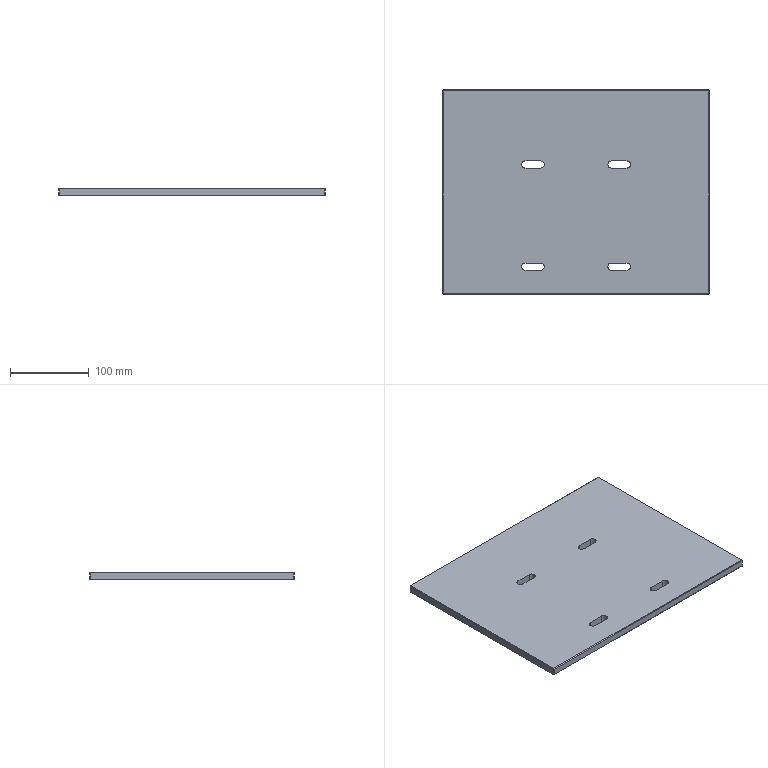Part | SolidWorks | features BaseBody 1 | 1 solid | 38 faces | box 340 x 260 x 10 mm | volume 873041 mm3 | plane 26 | cylinder 12 | commonest cylinder face diameters 9 x12
STEP:
#1=CARTESIAN_POINT('',(65.,-60.5,0.));
#2=VERTEX_POINT('',#1);
#3=CARTESIAN_POINT('',(69.5,-65.,0.));
#4=VERTEX_POINT('',#3);
#5=CARTESIAN_POINT('',(65.,-65.,0.));
#6=DIRECTION('',(0.,0.,-1.));
#7=DIRECTION('',(1.,0.,0.));
#8=AXIS2_PLACEMENT_3D('',#5,#6,#7);
#9=CIRCLE('',#8,4.5);
#10=EDGE_CURVE('',#2,#4,#9,.T.);
#11=ORIENTED_EDGE('',*,*,#10,.T.);
#12=CARTESIAN_POINT('',(69.5,-65.,10.));
#13=VERTEX_POINT('',#12);
#14=CARTESIAN_POINT('',(69.5,-65.,10.));
#15=DIRECTION('',(0.,0.,1.));
#16=VECTOR('',#15,1000.);
#17=LINE('',#14,#16);
#18=EDGE_CURVE('',#4,#13,#17,.T.);
#19=ORIENTED_EDGE('',*,*,#18,.T.);
#20=CARTESIAN_POINT('',(65.,-60.5,10.));
#21=VERTEX_POINT('',#20);
#22=CARTESIAN_POINT('',(65.,-65.,10.));
#23=DIRECTION('',(0.,0.,-1.));
#24=DIRECTION('',(1.,0.,0.));
#25=AXIS2_PLACEMENT_3D('',#22,#23,#24);
#26=CIRCLE('',#25,4.5);
#27=EDGE_CURVE('',#21,#13,#26,.T.);
#28=ORIENTED_EDGE('',*,*,#27,.F.);
#29=CARTESIAN_POINT('',(65.,-60.5,10.));
#30=DIRECTION('',(0.,0.,1.));
#31=VECTOR('',#30,1000.);
#32=LINE('',#29,#31);
#33=EDGE_CURVE('',#2,#21,#32,.T.);
#34=ORIENTED_EDGE('',*,*,#33,.F.);
#35=EDGE_LOOP('',(#11,#19,#28,#34));
#36=FACE_OUTER_BOUND('',#35,.T.);
#37=CARTESIAN_POINT('',(65.,-65.,10.));
#38=DIRECTION('',(0.,0.,1.));
#39=DIRECTION('',(1.,0.,0.));
#40=AXIS2_PLACEMENT_3D('',#37,#38,#39);
#41=CYLINDRICAL_SURFACE('',#40,4.5);
#42=ADVANCED_FACE('',(#36),#41,.F.);
#43=CARTESIAN_POINT('',(-45.,69.5,0.));
#44=VERTEX_POINT('',#43);
#45=CARTESIAN_POINT('',(-40.5,65.,0.));
#46=VERTEX_POINT('',#45);
#47=CARTESIAN_POINT('',(-45.,65.,0.));
#48=DIRECTION('',(0.,0.,-1.));
#49=DIRECTION('',(1.,0.,0.));
#50=AXIS2_PLACEMENT_3D('',#47,#48,#49);
#51=CIRCLE('',#50,4.5);
#52=EDGE_CURVE('',#44,#46,#51,.T.);
#53=ORIENTED_EDGE('',*,*,#52,.T.);
#54=CARTESIAN_POINT('',(-40.5,65.,10.));
#55=VERTEX_POINT('',#54);
#56=CARTESIAN_POINT('',(-40.5,65.,10.));
#57=DIRECTION('',(0.,0.,1.));
#58=VECTOR('',#57,1000.);
#59=LINE('',#56,#58);
#60=EDGE_CURVE('',#46,#55,#59,.T.);
#61=ORIENTED_EDGE('',*,*,#60,.T.);
#62=CARTESIAN_POINT('',(-45.,69.5,10.));
#63=VERTEX_POINT('',#62);
#64=CARTESIAN_POINT('',(-45.,65.,10.));
#65=DIRECTION('',(0.,0.,-1.));
#66=DIRECTION('',(1.,0.,0.));
#67=AXIS2_PLACEMENT_3D('',#64,#65,#66);
#68=CIRCLE('',#67,4.5);
#69=EDGE_CURVE('',#63,#55,#68,.T.);
#70=ORIENTED_EDGE('',*,*,#69,.F.);
#71=CARTESIAN_POINT('',(-45.,69.5,10.));
#72=DIRECTION('',(0.,0.,1.));
#73=VECTOR('',#72,1000.);
#74=LINE('',#71,#73);
#75=EDGE_CURVE('',#44,#63,#74,.T.);
#76=ORIENTED_EDGE('',*,*,#75,.F.);
#77=EDGE_LOOP('',(#53,#61,#70,#76));
#78=FACE_OUTER_BOUND('',#77,.T.);
#79=CARTESIAN_POINT('',(-45.,65.,10.));
#80=DIRECTION('',(0.,0.,1.));
#81=DIRECTION('',(1.,0.,0.));
#82=AXIS2_PLACEMENT_3D('',#79,#80,#81);
#83=CYLINDRICAL_SURFACE('',#82,4.5);
#84=ADVANCED_FACE('',(#78),#83,.F.);
#85=CARTESIAN_POINT('',(-45.,-60.5,0.));
#86=VERTEX_POINT('',#85);
#87=CARTESIAN_POINT('',(-40.5,-65.,0.));
#88=VERTEX_POINT('',#87);
#89=CARTESIAN_POINT('',(-45.,-65.,0.));
#90=DIRECTION('',(0.,0.,-1.));
#91=DIRECTION('',(1.,0.,0.));
#92=AXIS2_PLACEMENT_3D('',#89,#90,#91);
#93=CIRCLE('',#92,4.5);
#94=EDGE_CURVE('',#86,#88,#93,.T.);
#95=ORIENTED_EDGE('',*,*,#94,.T.);
#96=CARTESIAN_POINT('',(-40.5,-65.,10.));
#97=VERTEX_POINT('',#96);
#98=CARTESIAN_POINT('',(-40.5,-65.,10.));
#99=DIRECTION('',(0.,0.,1.));
#100=VECTOR('',#99,1000.);
#101=LINE('',#98,#100);
#102=EDGE_CURVE('',#88,#97,#101,.T.);
#103=ORIENTED_EDGE('',*,*,#102,.T.);
#104=CARTESIAN_POINT('',(-45.,-60.5,10.));
#105=VERTEX_POINT('',#104);
#106=CARTESIAN_POINT('',(-45.,-65.,10.));
#107=DIRECTION('',(0.,0.,-1.));
#108=DIRECTION('',(1.,0.,0.));
#109=AXIS2_PLACEMENT_3D('',#106,#107,#108);
#110=CIRCLE('',#109,4.5);
#111=EDGE_CURVE('',#105,#97,#110,.T.);
#112=ORIENTED_EDGE('',*,*,#111,.F.);
#113=CARTESIAN_POINT('',(-45.,-60.5,10.));
#114=DIRECTION('',(0.,0.,1.));
#115=VECTOR('',#114,1000.);
#116=LINE('',#113,#115);
#117=EDGE_CURVE('',#86,#105,#116,.T.);
#118=ORIENTED_EDGE('',*,*,#117,.F.);
#119=EDGE_LOOP('',(#95,#103,#112,#118));
#120=FACE_OUTER_BOUND('',#119,.T.);
#121=CARTESIAN_POINT('',(-45.,-65.,10.));
#122=DIRECTION('',(0.,0.,1.));
#123=DIRECTION('',(1.,0.,0.));
#124=AXIS2_PLACEMENT_3D('',#121,#122,#123);
#125=CYLINDRICAL_SURFACE('',#124,4.5);
#126=ADVANCED_FACE('',(#120),#125,.F.);
#127=CARTESIAN_POINT('',(65.,69.5,0.));
#128=VERTEX_POINT('',#127);
#129=CARTESIAN_POINT('',(69.5,65.,0.));
#130=VERTEX_POINT('',#129);
#131=CARTESIAN_POINT('',(65.,65.,0.));
#132=DIRECTION('',(0.,0.,-1.));
#133=DIRECTION('',(1.,0.,0.));
#134=AXIS2_PLACEMENT_3D('',#131,#132,#133);
#135=CIRCLE('',#134,4.5);
#136=EDGE_CURVE('',#128,#130,#135,.T.);
#137=ORIENTED_EDGE('',*,*,#136,.T.);
#138=CARTESIAN_POINT('',(69.5,65.,10.));
#139=VERTEX_POINT('',#138);
#140=CARTESIAN_POINT('',(69.5,65.,10.));
#141=DIRECTION('',(0.,0.,1.));
#142=VECTOR('',#141,1000.);
#143=LINE('',#140,#142);
#144=EDGE_CURVE('',#130,#139,#143,.T.);
#145=ORIENTED_EDGE('',*,*,#144,.T.);
#146=CARTESIAN_POINT('',(65.,69.5,10.));
#147=VERTEX_POINT('',#146);
#148=CARTESIAN_POINT('',(65.,65.,10.));
#149=DIRECTION('',(0.,0.,-1.));
#150=DIRECTION('',(1.,0.,0.));
#151=AXIS2_PLACEMENT_3D('',#148,#149,#150);
#152=CIRCLE('',#151,4.5);
#153=EDGE_CURVE('',#147,#139,#152,.T.);
#154=ORIENTED_EDGE('',*,*,#153,.F.);
#155=CARTESIAN_POINT('',(65.,69.5,10.));
#156=DIRECTION('',(0.,0.,1.));
#157=VECTOR('',#156,1000.);
#158=LINE('',#155,#157);
#159=EDGE_CURVE('',#128,#147,#158,.T.);
#160=ORIENTED_EDGE('',*,*,#159,.F.);
#161=EDGE_LOOP('',(#137,#145,#154,#160));
#162=FACE_OUTER_BOUND('',#161,.T.);
#163=CARTESIAN_POINT('',(65.,65.,10.));
#164=DIRECTION('',(0.,0.,1.));
#165=DIRECTION('',(1.,0.,0.));
#166=AXIS2_PLACEMENT_3D('',#163,#164,#165);
#167=CYLINDRICAL_SURFACE('',#166,4.5);
#168=ADVANCED_FACE('',(#162),#167,.F.);
#169=ORIENTED_EDGE('',*,*,#10,.F.);
#170=CARTESIAN_POINT('',(45.,-60.5,0.));
#171=VERTEX_POINT('',#170);
#172=CARTESIAN_POINT('',(0.,-60.5,0.));
#173=DIRECTION('',(1.,0.,0.));
#174=VECTOR('',#173,1000.);
#175=LINE('',#172,#174);
#176=EDGE_CURVE('',#171,#2,#175,.T.);
#177=ORIENTED_EDGE('',*,*,#176,.F.);
#178=CARTESIAN_POINT('',(45.,-69.5,0.));
#179=VERTEX_POINT('',#178);
#180=CARTESIAN_POINT('',(45.,-65.,0.));
#181=DIRECTION('',(0.,0.,-1.));
#182=DIRECTION('',(1.,0.,0.));
#183=AXIS2_PLACEMENT_3D('',#180,#181,#182);
#184=CIRCLE('',#183,4.5);
#185=EDGE_CURVE('',#179,#171,#184,.T.);
#186=ORIENTED_EDGE('',*,*,#185,.F.);
#187=CARTESIAN_POINT('',(65.,-69.5,0.));
#188=VERTEX_POINT('',#187);
#189=CARTESIAN_POINT('',(0.,-69.5,0.));
#190=DIRECTION('',(-1.,0.,0.));
#191=VECTOR('',#190,1000.);
#192=LINE('',#189,#191);
#193=EDGE_CURVE('',#188,#179,#192,.T.);
#194=ORIENTED_EDGE('',*,*,#193,.F.);
#195=CARTESIAN_POINT('',(65.,-65.,0.));
#196=DIRECTION('',(0.,0.,-1.));
#197=DIRECTION('',(1.,0.,0.));
#198=AXIS2_PLACEMENT_3D('',#195,#196,#197);
#199=CIRCLE('',#198,4.5);
#200=EDGE_CURVE('',#4,#188,#199,.T.);
#201=ORIENTED_EDGE('',*,*,#200,.F.);
#202=EDGE_LOOP('',(#169,#177,#186,#194,#201));
#203=FACE_BOUND('',#202,.T.);
#204=ORIENTED_EDGE('',*,*,#52,.F.);
#205=CARTESIAN_POINT('',(-65.,69.5,0.));
#206=VERTEX_POINT('',#205);
#207=CARTESIAN_POINT('',(0.,69.5,0.));
#208=DIRECTION('',(1.,0.,0.));
#209=VECTOR('',#208,1000.);
#210=LINE('',#207,#209);
#211=EDGE_CURVE('',#206,#44,#210,.T.);
#212=ORIENTED_EDGE('',*,*,#211,.F.);
#213=CARTESIAN_POINT('',(-65.,60.5,0.));
#214=VERTEX_POINT('',#213);
#215=CARTESIAN_POINT('',(-65.,65.,0.));
#216=DIRECTION('',(0.,0.,-1.));
#217=DIRECTION('',(1.,0.,0.));
#218=AXIS2_PLACEMENT_3D('',#215,#216,#217);
#219=CIRCLE('',#218,4.5);
#220=EDGE_CURVE('',#214,#206,#219,.T.);
#221=ORIENTED_EDGE('',*,*,#220,.F.);
#222=CARTESIAN_POINT('',(-45.,60.5,0.));
#223=VERTEX_POINT('',#222);
#224=CARTESIAN_POINT('',(0.,60.5,0.));
#225=DIRECTION('',(-1.,0.,0.));
#226=VECTOR('',#225,1000.);
#227=LINE('',#224,#226);
#228=EDGE_CURVE('',#223,#214,#227,.T.);
#229=ORIENTED_EDGE('',*,*,#228,.F.);
#230=CARTESIAN_POINT('',(-45.,65.,0.));
#231=DIRECTION('',(0.,0.,-1.));
#232=DIRECTION('',(1.,0.,0.));
#233=AXIS2_PLACEMENT_3D('',#230,#231,#232);
#234=CIRCLE('',#233,4.5);
#235=EDGE_CURVE('',#46,#223,#234,.T.);
#236=ORIENTED_EDGE('',*,*,#235,.F.);
#237=EDGE_LOOP('',(#204,#212,#221,#229,#236));
#238=FACE_BOUND('',#237,.T.);
#239=ORIENTED_EDGE('',*,*,#94,.F.);
#240=CARTESIAN_POINT('',(-65.,-60.5,0.));
#241=VERTEX_POINT('',#240);
#242=CARTESIAN_POINT('',(0.,-60.5,0.));
#243=DIRECTION('',(1.,0.,0.));
#244=VECTOR('',#243,1000.);
#245=LINE('',#242,#244);
#246=EDGE_CURVE('',#241,#86,#245,.T.);
#247=ORIENTED_EDGE('',*,*,#246,.F.);
#248=CARTESIAN_POINT('',(-65.,-69.5,0.));
#249=VERTEX_POINT('',#248);
#250=CARTESIAN_POINT('',(-65.,-65.,0.));
#251=DIRECTION('',(0.,0.,-1.));
#252=DIRECTION('',(1.,0.,0.));
#253=AXIS2_PLACEMENT_3D('',#250,#251,#252);
#254=CIRCLE('',#253,4.5);
#255=EDGE_CURVE('',#249,#241,#254,.T.);
#256=ORIENTED_EDGE('',*,*,#255,.F.);
#257=CARTESIAN_POINT('',(-45.,-69.5,0.));
#258=VERTEX_POINT('',#257);
#259=CARTESIAN_POINT('',(0.,-69.5,0.));
#260=DIRECTION('',(-1.,0.,0.));
#261=VECTOR('',#260,1000.);
#262=LINE('',#259,#261);
#263=EDGE_CURVE('',#258,#249,#262,.T.);
#264=ORIENTED_EDGE('',*,*,#263,.F.);
#265=CARTESIAN_POINT('',(-45.,-65.,0.));
#266=DIRECTION('',(0.,0.,-1.));
#267=DIRECTION('',(1.,0.,0.));
#268=AXIS2_PLACEMENT_3D('',#265,#266,#267);
#269=CIRCLE('',#268,4.5);
#270=EDGE_CURVE('',#88,#258,#269,.T.);
#271=ORIENTED_EDGE('',*,*,#270,.F.);
#272=EDGE_LOOP('',(#239,#247,#256,#264,#271));
#273=FACE_BOUND('',#272,.T.);
#274=ORIENTED_EDGE('',*,*,#136,.F.);
#275=CARTESIAN_POINT('',(45.,69.5,0.));
#276=VERTEX_POINT('',#275);
#277=CARTESIAN_POINT('',(0.,69.5,0.));
#278=DIRECTION('',(1.,0.,0.));
#279=VECTOR('',#278,1000.);
#280=LINE('',#277,#279);
#281=EDGE_CURVE('',#276,#128,#280,.T.);
#282=ORIENTED_EDGE('',*,*,#281,.F.);
#283=CARTESIAN_POINT('',(45.,60.5,0.));
#284=VERTEX_POINT('',#283);
#285=CARTESIAN_POINT('',(45.,65.,0.));
#286=DIRECTION('',(0.,0.,-1.));
#287=DIRECTION('',(1.,0.,0.));
#288=AXIS2_PLACEMENT_3D('',#285,#286,#287);
#289=CIRCLE('',#288,4.5);
#290=EDGE_CURVE('',#284,#276,#289,.T.);
#291=ORIENTED_EDGE('',*,*,#290,.F.);
#292=CARTESIAN_POINT('',(65.,60.5,0.));
#293=VERTEX_POINT('',#292);
#294=CARTESIAN_POINT('',(0.,60.5,0.));
#295=DIRECTION('',(-1.,0.,0.));
#296=VECTOR('',#295,1000.);
#297=LINE('',#294,#296);
#298=EDGE_CURVE('',#293,#284,#297,.T.);
#299=ORIENTED_EDGE('',*,*,#298,.F.);
#300=CARTESIAN_POINT('',(65.,65.,0.));
#301=DIRECTION('',(0.,0.,-1.));
#302=DIRECTION('',(1.,0.,0.));
#303=AXIS2_PLACEMENT_3D('',#300,#301,#302);
#304=CIRCLE('',#303,4.5);
#305=EDGE_CURVE('',#130,#293,#304,.T.);
#306=ORIENTED_EDGE('',*,*,#305,.F.);
#307=EDGE_LOOP('',(#274,#282,#291,#299,#306));
#308=FACE_BOUND('',#307,.T.);
#309=CARTESIAN_POINT('',(169.,-99.,0.));
#310=VERTEX_POINT('',#309);
#311=CARTESIAN_POINT('',(169.,159.,0.));
#312=VERTEX_POINT('',#311);
#313=CARTESIAN_POINT('',(169.,0.,0.));
#314=DIRECTION('',(0.,1.,0.));
#315=VECTOR('',#314,1000.);
#316=LINE('',#313,#315);
#317=EDGE_CURVE('',#310,#312,#316,.T.);
#318=ORIENTED_EDGE('',*,*,#317,.F.);
#319=CARTESIAN_POINT('',(-169.,-99.,0.));
#320=VERTEX_POINT('',#319);
#321=CARTESIAN_POINT('',(0.,-99.,0.));
#322=DIRECTION('',(1.,0.,0.));
#323=VECTOR('',#322,1000.);
#324=LINE('',#321,#323);
#325=EDGE_CURVE('',#320,#310,#324,.T.);
#326=ORIENTED_EDGE('',*,*,#325,.F.);
#327=CARTESIAN_POINT('',(-169.,159.,0.));
#328=VERTEX_POINT('',#327);
#329=CARTESIAN_POINT('',(-169.,0.,0.));
#330=DIRECTION('',(0.,-1.,0.));
#331=VECTOR('',#330,1000.);
#332=LINE('',#329,#331);
#333=EDGE_CURVE('',#328,#320,#332,.T.);
#334=ORIENTED_EDGE('',*,*,#333,.F.);
#335=CARTESIAN_POINT('',(0.,159.,0.));
#336=DIRECTION('',(-1.,0.,0.));
#337=VECTOR('',#336,1000.);
#338=LINE('',#335,#337);
#339=EDGE_CURVE('',#312,#328,#338,.T.);
#340=ORIENTED_EDGE('',*,*,#339,.F.);
#341=EDGE_LOOP('',(#318,#326,#334,#340));
#342=FACE_OUTER_BOUND('',#341,.T.);
#343=CARTESIAN_POINT('',(0.,0.,0.));
#344=DIRECTION('',(0.,0.,1.));
#345=DIRECTION('',(1.,0.,0.));
#346=AXIS2_PLACEMENT_3D('',#343,#344,#345);
#347=PLANE('',#346);
#348=ADVANCED_FACE('',(#203,#238,#273,#308,#342),#347,.F.);
#349=CARTESIAN_POINT('',(65.,-69.5,10.));
#350=VERTEX_POINT('',#349);
#351=CARTESIAN_POINT('',(45.,-69.5,10.));
#352=VERTEX_POINT('',#351);
#353=CARTESIAN_POINT('',(45.,-69.5,10.));
#354=DIRECTION('',(-1.,0.,0.));
#355=VECTOR('',#354,1000.);
#356=LINE('',#353,#355);
#357=EDGE_CURVE('',#350,#352,#356,.T.);
#358=ORIENTED_EDGE('',*,*,#357,.F.);
#359=CARTESIAN_POINT('',(65.,-69.5,10.));
#360=DIRECTION('',(0.,0.,1.));
#361=VECTOR('',#360,1000.);
#362=LINE('',#359,#361);
#363=EDGE_CURVE('',#188,#350,#362,.T.);
#364=ORIENTED_EDGE('',*,*,#363,.F.);
#365=ORIENTED_EDGE('',*,*,#193,.T.);
#366=CARTESIAN_POINT('',(45.,-69.5,10.));
#367=DIRECTION('',(0.,0.,-1.));
#368=VECTOR('',#367,1000.);
#369=LINE('',#366,#368);
#370=EDGE_CURVE('',#352,#179,#369,.T.);
#371=ORIENTED_EDGE('',*,*,#370,.F.);
#372=EDGE_LOOP('',(#358,#364,#365,#371));
#373=FACE_OUTER_BOUND('',#372,.T.);
#374=CARTESIAN_POINT('',(45.,-69.5,10.));
#375=DIRECTION('',(0.,-1.,0.));
#376=DIRECTION('',(0.,0.,-1.));
#377=AXIS2_PLACEMENT_3D('',#374,#375,#376);
#378=PLANE('',#377);
#379=ADVANCED_FACE('',(#373),#378,.F.);
#380=ORIENTED_EDGE('',*,*,#18,.F.);
#381=ORIENTED_EDGE('',*,*,#200,.T.);
#382=ORIENTED_EDGE('',*,*,#363,.T.);
#383=CARTESIAN_POINT('',(65.,-65.,10.));
#384=DIRECTION('',(0.,0.,-1.));
#385=DIRECTION('',(1.,0.,0.));
#386=AXIS2_PLACEMENT_3D('',#383,#384,#385);
#387=CIRCLE('',#386,4.5);
#388=EDGE_CURVE('',#13,#350,#387,.T.);
#389=ORIENTED_EDGE('',*,*,#388,.F.);
#390=EDGE_LOOP('',(#380,#381,#382,#389));
#391=FACE_OUTER_BOUND('',#390,.T.);
#392=CARTESIAN_POINT('',(65.,-65.,10.));
#393=DIRECTION('',(0.,0.,1.));
#394=DIRECTION('',(1.,0.,0.));
#395=AXIS2_PLACEMENT_3D('',#392,#393,#394);
#396=CYLINDRICAL_SURFACE('',#395,4.5);
#397=ADVANCED_FACE('',(#391),#396,.F.);
#398=CARTESIAN_POINT('',(45.,-60.5,10.));
#399=VERTEX_POINT('',#398);
#400=CARTESIAN_POINT('',(65.,-60.5,10.));
#401=DIRECTION('',(1.,0.,0.));
#402=VECTOR('',#401,1000.);
#403=LINE('',#400,#402);
#404=EDGE_CURVE('',#399,#21,#403,.T.);
#405=ORIENTED_EDGE('',*,*,#404,.F.);
#406=CARTESIAN_POINT('',(45.,-60.5,10.));
#407=DIRECTION('',(0.,0.,1.));
#408=VECTOR('',#407,1000.);
#409=LINE('',#406,#408);
#410=EDGE_CURVE('',#171,#399,#409,.T.);
#411=ORIENTED_EDGE('',*,*,#410,.F.);
#412=ORIENTED_EDGE('',*,*,#176,.T.);
#413=ORIENTED_EDGE('',*,*,#33,.T.);
#414=EDGE_LOOP('',(#405,#411,#412,#413));
#415=FACE_OUTER_BOUND('',#414,.T.);
#416=CARTESIAN_POINT('',(65.,-60.5,10.));
#417=DIRECTION('',(0.,1.,0.));
#418=DIRECTION('',(0.,0.,1.));
#419=AXIS2_PLACEMENT_3D('',#416,#417,#418);
#420=PLANE('',#419);
#421=ADVANCED_FACE('',(#415),#420,.F.);
#422=CARTESIAN_POINT('',(45.,-65.,10.));
#423=DIRECTION('',(0.,0.,-1.));
#424=DIRECTION('',(1.,0.,0.));
#425=AXIS2_PLACEMENT_3D('',#422,#423,#424);
#426=CIRCLE('',#425,4.5);
#427=EDGE_CURVE('',#352,#399,#426,.T.);
#428=ORIENTED_EDGE('',*,*,#427,.F.);
#429=ORIENTED_EDGE('',*,*,#370,.T.);
#430=ORIENTED_EDGE('',*,*,#185,.T.);
#431=ORIENTED_EDGE('',*,*,#410,.T.);
#432=EDGE_LOOP('',(#428,#429,#430,#431));
#433=FACE_OUTER_BOUND('',#432,.T.);
#434=CARTESIAN_POINT('',(45.,-65.,10.));
#435=DIRECTION('',(0.,0.,1.));
#436=DIRECTION('',(1.,0.,0.));
#437=AXIS2_PLACEMENT_3D('',#434,#435,#436);
#438=CYLINDRICAL_SURFACE('',#437,4.5);
#439=ADVANCED_FACE('',(#433),#438,.F.);
#440=CARTESIAN_POINT('',(-45.,60.5,10.));
#441=VERTEX_POINT('',#440);
#442=CARTESIAN_POINT('',(-65.,60.5,10.));
#443=VERTEX_POINT('',#442);
#444=CARTESIAN_POINT('',(-65.,60.5,10.));
#445=DIRECTION('',(-1.,0.,0.));
#446=VECTOR('',#445,1000.);
#447=LINE('',#444,#446);
#448=EDGE_CURVE('',#441,#443,#447,.T.);
#449=ORIENTED_EDGE('',*,*,#448,.F.);
#450=CARTESIAN_POINT('',(-45.,60.5,10.));
#451=DIRECTION('',(0.,0.,1.));
#452=VECTOR('',#451,1000.);
#453=LINE('',#450,#452);
#454=EDGE_CURVE('',#223,#441,#453,.T.);
#455=ORIENTED_EDGE('',*,*,#454,.F.);
#456=ORIENTED_EDGE('',*,*,#228,.T.);
#457=CARTESIAN_POINT('',(-65.,60.5,10.));
#458=DIRECTION('',(0.,0.,-1.));
#459=VECTOR('',#458,1000.);
#460=LINE('',#457,#459);
#461=EDGE_CURVE('',#443,#214,#460,.T.);
#462=ORIENTED_EDGE('',*,*,#461,.F.);
#463=EDGE_LOOP('',(#449,#455,#456,#462));
#464=FACE_OUTER_BOUND('',#463,.T.);
#465=CARTESIAN_POINT('',(-65.,60.5,10.));
#466=DIRECTION('',(0.,-1.,0.));
#467=DIRECTION('',(0.,0.,-1.));
#468=AXIS2_PLACEMENT_3D('',#465,#466,#467);
#469=PLANE('',#468);
#470=ADVANCED_FACE('',(#464),#469,.F.);
#471=ORIENTED_EDGE('',*,*,#60,.F.);
#472=ORIENTED_EDGE('',*,*,#235,.T.);
#473=ORIENTED_EDGE('',*,*,#454,.T.);
#474=CARTESIAN_POINT('',(-45.,65.,10.));
#475=DIRECTION('',(0.,0.,-1.));
#476=DIRECTION('',(1.,0.,0.));
#477=AXIS2_PLACEMENT_3D('',#474,#475,#476);
#478=CIRCLE('',#477,4.5);
#479=EDGE_CURVE('',#55,#441,#478,.T.);
#480=ORIENTED_EDGE('',*,*,#479,.F.);
#481=EDGE_LOOP('',(#471,#472,#473,#480));
#482=FACE_OUTER_BOUND('',#481,.T.);
#483=CARTESIAN_POINT('',(-45.,65.,10.));
#484=DIRECTION('',(0.,0.,1.));
#485=DIRECTION('',(1.,0.,0.));
#486=AXIS2_PLACEMENT_3D('',#483,#484,#485);
#487=CYLINDRICAL_SURFACE('',#486,4.5);
#488=ADVANCED_FACE('',(#482),#487,.F.);
#489=CARTESIAN_POINT('',(-65.,69.5,10.));
#490=VERTEX_POINT('',#489);
#491=CARTESIAN_POINT('',(-45.,69.5,10.));
#492=DIRECTION('',(1.,0.,0.));
#493=VECTOR('',#492,1000.);
#494=LINE('',#491,#493);
#495=EDGE_CURVE('',#490,#63,#494,.T.);
#496=ORIENTED_EDGE('',*,*,#495,.F.);
#497=CARTESIAN_POINT('',(-65.,69.5,10.));
#498=DIRECTION('',(0.,0.,1.));
#499=VECTOR('',#498,1000.);
#500=LINE('',#497,#499);
#501=EDGE_CURVE('',#206,#490,#500,.T.);
#502=ORIENTED_EDGE('',*,*,#501,.F.);
#503=ORIENTED_EDGE('',*,*,#211,.T.);
#504=ORIENTED_EDGE('',*,*,#75,.T.);
#505=EDGE_LOOP('',(#496,#502,#503,#504));
#506=FACE_OUTER_BOUND('',#505,.T.);
#507=CARTESIAN_POINT('',(-45.,69.5,10.));
#508=DIRECTION('',(0.,1.,0.));
#509=DIRECTION('',(0.,0.,1.));
#510=AXIS2_PLACEMENT_3D('',#507,#508,#509);
#511=PLANE('',#510);
#512=ADVANCED_FACE('',(#506),#511,.F.);
#513=CARTESIAN_POINT('',(-65.,65.,10.));
#514=DIRECTION('',(0.,0.,-1.));
#515=DIRECTION('',(1.,0.,0.));
#516=AXIS2_PLACEMENT_3D('',#513,#514,#515);
#517=CIRCLE('',#516,4.5);
#518=EDGE_CURVE('',#443,#490,#517,.T.);
#519=ORIENTED_EDGE('',*,*,#518,.F.);
#520=ORIENTED_EDGE('',*,*,#461,.T.);
#521=ORIENTED_EDGE('',*,*,#220,.T.);
#522=ORIENTED_EDGE('',*,*,#501,.T.);
#523=EDGE_LOOP('',(#519,#520,#521,#522));
#524=FACE_OUTER_BOUND('',#523,.T.);
#525=CARTESIAN_POINT('',(-65.,65.,10.));
#526=DIRECTION('',(0.,0.,1.));
#527=DIRECTION('',(1.,0.,0.));
#528=AXIS2_PLACEMENT_3D('',#525,#526,#527);
#529=CYLINDRICAL_SURFACE('',#528,4.5);
#530=ADVANCED_FACE('',(#524),#529,.F.);
#531=CARTESIAN_POINT('',(-45.,-69.5,10.));
#532=VERTEX_POINT('',#531);
#533=CARTESIAN_POINT('',(-65.,-69.5,10.));
#534=VERTEX_POINT('',#533);
#535=CARTESIAN_POINT('',(-65.,-69.5,10.));
#536=DIRECTION('',(-1.,0.,0.));
#537=VECTOR('',#536,1000.);
#538=LINE('',#535,#537);
#539=EDGE_CURVE('',#532,#534,#538,.T.);
#540=ORIENTED_EDGE('',*,*,#539,.F.);
#541=CARTESIAN_POINT('',(-45.,-69.5,10.));
#542=DIRECTION('',(0.,0.,1.));
#543=VECTOR('',#542,1000.);
#544=LINE('',#541,#543);
#545=EDGE_CURVE('',#258,#532,#544,.T.);
#546=ORIENTED_EDGE('',*,*,#545,.F.);
#547=ORIENTED_EDGE('',*,*,#263,.T.);
#548=CARTESIAN_POINT('',(-65.,-69.5,10.));
#549=DIRECTION('',(0.,0.,-1.));
#550=VECTOR('',#549,1000.);
#551=LINE('',#548,#550);
#552=EDGE_CURVE('',#534,#249,#551,.T.);
#553=ORIENTED_EDGE('',*,*,#552,.F.);
#554=EDGE_LOOP('',(#540,#546,#547,#553));
#555=FACE_OUTER_BOUND('',#554,.T.);
#556=CARTESIAN_POINT('',(-65.,-69.5,10.));
#557=DIRECTION('',(0.,-1.,0.));
#558=DIRECTION('',(0.,0.,-1.));
#559=AXIS2_PLACEMENT_3D('',#556,#557,#558);
#560=PLANE('',#559);
#561=ADVANCED_FACE('',(#555),#560,.F.);
#562=ORIENTED_EDGE('',*,*,#102,.F.);
#563=ORIENTED_EDGE('',*,*,#270,.T.);
#564=ORIENTED_EDGE('',*,*,#545,.T.);
#565=CARTESIAN_POINT('',(-45.,-65.,10.));
#566=DIRECTION('',(0.,0.,-1.));
#567=DIRECTION('',(1.,0.,0.));
#568=AXIS2_PLACEMENT_3D('',#565,#566,#567);
#569=CIRCLE('',#568,4.5);
#570=EDGE_CURVE('',#97,#532,#569,.T.);
#571=ORIENTED_EDGE('',*,*,#570,.F.);
#572=EDGE_LOOP('',(#562,#563,#564,#571));
#573=FACE_OUTER_BOUND('',#572,.T.);
#574=CARTESIAN_POINT('',(-45.,-65.,10.));
#575=DIRECTION('',(0.,0.,1.));
#576=DIRECTION('',(1.,0.,0.));
#577=AXIS2_PLACEMENT_3D('',#574,#575,#576);
#578=CYLINDRICAL_SURFACE('',#577,4.5);
#579=ADVANCED_FACE('',(#573),#578,.F.);
#580=CARTESIAN_POINT('',(-65.,-60.5,10.));
#581=VERTEX_POINT('',#580);
#582=CARTESIAN_POINT('',(-45.,-60.5,10.));
#583=DIRECTION('',(1.,0.,0.));
#584=VECTOR('',#583,1000.);
#585=LINE('',#582,#584);
#586=EDGE_CURVE('',#581,#105,#585,.T.);
#587=ORIENTED_EDGE('',*,*,#586,.F.);
#588=CARTESIAN_POINT('',(-65.,-60.5,10.));
#589=DIRECTION('',(0.,0.,1.));
#590=VECTOR('',#589,1000.);
#591=LINE('',#588,#590);
#592=EDGE_CURVE('',#241,#581,#591,.T.);
#593=ORIENTED_EDGE('',*,*,#592,.F.);
#594=ORIENTED_EDGE('',*,*,#246,.T.);
#595=ORIENTED_EDGE('',*,*,#117,.T.);
#596=EDGE_LOOP('',(#587,#593,#594,#595));
#597=FACE_OUTER_BOUND('',#596,.T.);
#598=CARTESIAN_POINT('',(-45.,-60.5,10.));
#599=DIRECTION('',(0.,1.,0.));
#600=DIRECTION('',(0.,0.,1.));
#601=AXIS2_PLACEMENT_3D('',#598,#599,#600);
#602=PLANE('',#601);
#603=ADVANCED_FACE('',(#597),#602,.F.);
#604=CARTESIAN_POINT('',(-65.,-65.,10.));
#605=DIRECTION('',(0.,0.,-1.));
#606=DIRECTION('',(1.,0.,0.));
#607=AXIS2_PLACEMENT_3D('',#604,#605,#606);
#608=CIRCLE('',#607,4.5);
#609=EDGE_CURVE('',#534,#581,#608,.T.);
#610=ORIENTED_EDGE('',*,*,#609,.F.);
#611=ORIENTED_EDGE('',*,*,#552,.T.);
#612=ORIENTED_EDGE('',*,*,#255,.T.);
#613=ORIENTED_EDGE('',*,*,#592,.T.);
#614=EDGE_LOOP('',(#610,#611,#612,#613));
#615=FACE_OUTER_BOUND('',#614,.T.);
#616=CARTESIAN_POINT('',(-65.,-65.,10.));
#617=DIRECTION('',(0.,0.,1.));
#618=DIRECTION('',(1.,0.,0.));
#619=AXIS2_PLACEMENT_3D('',#616,#617,#618);
#620=CYLINDRICAL_SURFACE('',#619,4.5);
#621=ADVANCED_FACE('',(#615),#620,.F.);
#622=CARTESIAN_POINT('',(65.,60.5,10.));
#623=VERTEX_POINT('',#622);
#624=CARTESIAN_POINT('',(45.,60.5,10.));
#625=VERTEX_POINT('',#624);
#626=CARTESIAN_POINT('',(45.,60.5,10.));
#627=DIRECTION('',(-1.,0.,0.));
#628=VECTOR('',#627,1000.);
#629=LINE('',#626,#628);
#630=EDGE_CURVE('',#623,#625,#629,.T.);
#631=ORIENTED_EDGE('',*,*,#630,.F.);
#632=CARTESIAN_POINT('',(65.,60.5,10.));
#633=DIRECTION('',(0.,0.,1.));
#634=VECTOR('',#633,1000.);
#635=LINE('',#632,#634);
#636=EDGE_CURVE('',#293,#623,#635,.T.);
#637=ORIENTED_EDGE('',*,*,#636,.F.);
#638=ORIENTED_EDGE('',*,*,#298,.T.);
#639=CARTESIAN_POINT('',(45.,60.5,10.));
#640=DIRECTION('',(0.,0.,-1.));
#641=VECTOR('',#640,1000.);
#642=LINE('',#639,#641);
#643=EDGE_CURVE('',#625,#284,#642,.T.);
#644=ORIENTED_EDGE('',*,*,#643,.F.);
#645=EDGE_LOOP('',(#631,#637,#638,#644));
#646=FACE_OUTER_BOUND('',#645,.T.);
#647=CARTESIAN_POINT('',(45.,60.5,10.));
#648=DIRECTION('',(0.,-1.,0.));
#649=DIRECTION('',(0.,0.,-1.));
#650=AXIS2_PLACEMENT_3D('',#647,#648,#649);
#651=PLANE('',#650);
#652=ADVANCED_FACE('',(#646),#651,.F.);
#653=ORIENTED_EDGE('',*,*,#144,.F.);
#654=ORIENTED_EDGE('',*,*,#305,.T.);
#655=ORIENTED_EDGE('',*,*,#636,.T.);
#656=CARTESIAN_POINT('',(65.,65.,10.));
#657=DIRECTION('',(0.,0.,-1.));
#658=DIRECTION('',(1.,0.,0.));
#659=AXIS2_PLACEMENT_3D('',#656,#657,#658);
#660=CIRCLE('',#659,4.5);
#661=EDGE_CURVE('',#139,#623,#660,.T.);
#662=ORIENTED_EDGE('',*,*,#661,.F.);
#663=EDGE_LOOP('',(#653,#654,#655,#662));
#664=FACE_OUTER_BOUND('',#663,.T.);
#665=CARTESIAN_POINT('',(65.,65.,10.));
#666=DIRECTION('',(0.,0.,1.));
#667=DIRECTION('',(1.,0.,0.));
#668=AXIS2_PLACEMENT_3D('',#665,#666,#667);
#669=CYLINDRICAL_SURFACE('',#668,4.5);
#670=ADVANCED_FACE('',(#664),#669,.F.);
#671=CARTESIAN_POINT('',(45.,69.5,10.));
#672=VERTEX_POINT('',#671);
#673=CARTESIAN_POINT('',(65.,69.5,10.));
#674=DIRECTION('',(1.,0.,0.));
#675=VECTOR('',#674,1000.);
#676=LINE('',#673,#675);
#677=EDGE_CURVE('',#672,#147,#676,.T.);
#678=ORIENTED_EDGE('',*,*,#677,.F.);
#679=CARTESIAN_POINT('',(45.,69.5,10.));
#680=DIRECTION('',(0.,0.,1.));
#681=VECTOR('',#680,1000.);
#682=LINE('',#679,#681);
#683=EDGE_CURVE('',#276,#672,#682,.T.);
#684=ORIENTED_EDGE('',*,*,#683,.F.);
#685=ORIENTED_EDGE('',*,*,#281,.T.);
#686=ORIENTED_EDGE('',*,*,#159,.T.);
#687=EDGE_LOOP('',(#678,#684,#685,#686));
#688=FACE_OUTER_BOUND('',#687,.T.);
#689=CARTESIAN_POINT('',(65.,69.5,10.));
#690=DIRECTION('',(0.,1.,0.));
#691=DIRECTION('',(0.,0.,1.));
#692=AXIS2_PLACEMENT_3D('',#689,#690,#691);
#693=PLANE('',#692);
#694=ADVANCED_FACE('',(#688),#693,.F.);
#695=CARTESIAN_POINT('',(45.,65.,10.));
#696=DIRECTION('',(0.,0.,-1.));
#697=DIRECTION('',(1.,0.,0.));
#698=AXIS2_PLACEMENT_3D('',#695,#696,#697);
#699=CIRCLE('',#698,4.5);
#700=EDGE_CURVE('',#625,#672,#699,.T.);
#701=ORIENTED_EDGE('',*,*,#700,.F.);
#702=ORIENTED_EDGE('',*,*,#643,.T.);
#703=ORIENTED_EDGE('',*,*,#290,.T.);
#704=ORIENTED_EDGE('',*,*,#683,.T.);
#705=EDGE_LOOP('',(#701,#702,#703,#704));
#706=FACE_OUTER_BOUND('',#705,.T.);
#707=CARTESIAN_POINT('',(45.,65.,10.));
#708=DIRECTION('',(0.,0.,1.));
#709=DIRECTION('',(1.,0.,0.));
#710=AXIS2_PLACEMENT_3D('',#707,#708,#709);
#711=CYLINDRICAL_SURFACE('',#710,4.5);
#712=ADVANCED_FACE('',(#706),#711,.F.);
#713=CARTESIAN_POINT('',(-169.,160.,1.));
#714=VERTEX_POINT('',#713);
#715=CARTESIAN_POINT('',(-169.5,159.5,0.5));
#716=VERTEX_POINT('',#715);
#717=CARTESIAN_POINT('',(-169.,160.,1.));
#718=DIRECTION('',(-0.5774,-0.5774,-0.5774));
#719=VECTOR('',#718,1000.);
#720=LINE('',#717,#719);
#721=EDGE_CURVE('',#714,#716,#720,.T.);
#722=ORIENTED_EDGE('',*,*,#721,.F.);
#723=CARTESIAN_POINT('',(169.,160.,1.));
#724=VERTEX_POINT('',#723);
#725=CARTESIAN_POINT('',(0.,160.,1.));
#726=DIRECTION('',(1.,0.,0.));
#727=VECTOR('',#726,1000.);
#728=LINE('',#725,#727);
#729=EDGE_CURVE('',#714,#724,#728,.T.);
#730=ORIENTED_EDGE('',*,*,#729,.T.);
#731=CARTESIAN_POINT('',(169.5,159.5,0.5));
#732=VERTEX_POINT('',#731);
#733=CARTESIAN_POINT('',(169.5,159.5,0.5));
#734=DIRECTION('',(-0.5774,0.5774,0.5774));
#735=VECTOR('',#734,1000.);
#736=LINE('',#733,#735);
#737=EDGE_CURVE('',#732,#724,#736,.T.);
#738=ORIENTED_EDGE('',*,*,#737,.F.);
#739=CARTESIAN_POINT('',(169.5,159.5,0.5));
#740=DIRECTION('',(-0.5774,-0.5774,-0.5774));
#741=VECTOR('',#740,1000.);
#742=LINE('',#739,#741);
#743=EDGE_CURVE('',#732,#312,#742,.T.);
#744=ORIENTED_EDGE('',*,*,#743,.T.);
#745=ORIENTED_EDGE('',*,*,#339,.T.);
#746=CARTESIAN_POINT('',(-169.,159.,0.));
#747=DIRECTION('',(-0.5774,0.5774,0.5774));
#748=VECTOR('',#747,1000.);
#749=LINE('',#746,#748);
#750=EDGE_CURVE('',#328,#716,#749,.T.);
#751=ORIENTED_EDGE('',*,*,#750,.T.);
#752=EDGE_LOOP('',(#722,#730,#738,#744,#745,#751));
#753=FACE_OUTER_BOUND('',#752,.T.);
#754=CARTESIAN_POINT('',(0.,159.5,0.5));
#755=DIRECTION('',(0.,0.7071,-0.7071));
#756=DIRECTION('',(0.,0.7071,0.7071));
#757=AXIS2_PLACEMENT_3D('',#754,#755,#756);
#758=PLANE('',#757);
#759=ADVANCED_FACE('',(#753),#758,.T.);
#760=CARTESIAN_POINT('',(169.5,-99.5,0.5));
#761=VERTEX_POINT('',#760);
#762=CARTESIAN_POINT('',(169.5,-99.5,0.5));
#763=DIRECTION('',(-0.5774,0.5774,-0.5774));
#764=VECTOR('',#763,1000.);
#765=LINE('',#762,#764);
#766=EDGE_CURVE('',#761,#310,#765,.T.);
#767=ORIENTED_EDGE('',*,*,#766,.T.);
#768=ORIENTED_EDGE('',*,*,#317,.T.);
#769=ORIENTED_EDGE('',*,*,#743,.F.);
#770=CARTESIAN_POINT('',(170.,159.,1.));
#771=VERTEX_POINT('',#770);
#772=CARTESIAN_POINT('',(170.,159.,1.));
#773=DIRECTION('',(-0.5774,0.5774,-0.5774));
#774=VECTOR('',#773,1000.);
#775=LINE('',#772,#774);
#776=EDGE_CURVE('',#771,#732,#775,.T.);
#777=ORIENTED_EDGE('',*,*,#776,.F.);
#778=CARTESIAN_POINT('',(170.,-99.,1.));
#779=VERTEX_POINT('',#778);
#780=CARTESIAN_POINT('',(170.,30.,1.));
#781=DIRECTION('',(0.,-1.,0.));
#782=VECTOR('',#781,1000.);
#783=LINE('',#780,#782);
#784=EDGE_CURVE('',#771,#779,#783,.T.);
#785=ORIENTED_EDGE('',*,*,#784,.T.);
#786=CARTESIAN_POINT('',(169.5,-99.5,0.5));
#787=DIRECTION('',(0.5774,0.5774,0.5774));
#788=VECTOR('',#787,1000.);
#789=LINE('',#786,#788);
#790=EDGE_CURVE('',#761,#779,#789,.T.);
#791=ORIENTED_EDGE('',*,*,#790,.F.);
#792=EDGE_LOOP('',(#767,#768,#769,#777,#785,#791));
#793=FACE_OUTER_BOUND('',#792,.T.);
#794=CARTESIAN_POINT('',(169.5,30.,0.5));
#795=DIRECTION('',(0.7071,0.,-0.7071));
#796=DIRECTION('',(-0.7071,0.,-0.7071));
#797=AXIS2_PLACEMENT_3D('',#794,#795,#796);
#798=PLANE('',#797);
#799=ADVANCED_FACE('',(#793),#798,.T.);
#800=CARTESIAN_POINT('',(-169.5,-99.5,0.5));
#801=VERTEX_POINT('',#800);
#802=CARTESIAN_POINT('',(-169.5,-99.5,0.5));
#803=DIRECTION('',(0.5774,0.5774,-0.5774));
#804=VECTOR('',#803,1000.);
#805=LINE('',#802,#804);
#806=EDGE_CURVE('',#801,#320,#805,.T.);
#807=ORIENTED_EDGE('',*,*,#806,.T.);
#808=ORIENTED_EDGE('',*,*,#325,.T.);
#809=ORIENTED_EDGE('',*,*,#766,.F.);
#810=CARTESIAN_POINT('',(169.,-100.,1.));
#811=VERTEX_POINT('',#810);
#812=CARTESIAN_POINT('',(169.,-100.,1.));
#813=DIRECTION('',(0.5774,0.5774,-0.5774));
#814=VECTOR('',#813,1000.);
#815=LINE('',#812,#814);
#816=EDGE_CURVE('',#811,#761,#815,.T.);
#817=ORIENTED_EDGE('',*,*,#816,.F.);
#818=CARTESIAN_POINT('',(-169.,-100.,1.));
#819=VERTEX_POINT('',#818);
#820=CARTESIAN_POINT('',(0.,-100.,1.));
#821=DIRECTION('',(-1.,0.,0.));
#822=VECTOR('',#821,1000.);
#823=LINE('',#820,#822);
#824=EDGE_CURVE('',#811,#819,#823,.T.);
#825=ORIENTED_EDGE('',*,*,#824,.T.);
#826=CARTESIAN_POINT('',(-169.5,-99.5,0.5));
#827=DIRECTION('',(0.5774,-0.5774,0.5774));
#828=VECTOR('',#827,1000.);
#829=LINE('',#826,#828);
#830=EDGE_CURVE('',#801,#819,#829,.T.);
#831=ORIENTED_EDGE('',*,*,#830,.F.);
#832=EDGE_LOOP('',(#807,#808,#809,#817,#825,#831));
#833=FACE_OUTER_BOUND('',#832,.T.);
#834=CARTESIAN_POINT('',(0.,-99.5,0.5));
#835=DIRECTION('',(0.,-0.7071,-0.7071));
#836=DIRECTION('',(0.,0.7071,-0.7071));
#837=AXIS2_PLACEMENT_3D('',#834,#835,#836);
#838=PLANE('',#837);
#839=ADVANCED_FACE('',(#833),#838,.T.);
#840=CARTESIAN_POINT('',(-170.,-99.,1.));
#841=VERTEX_POINT('',#840);
#842=CARTESIAN_POINT('',(-170.,-99.,1.));
#843=DIRECTION('',(0.5774,-0.5774,-0.5774));
#844=VECTOR('',#843,1000.);
#845=LINE('',#842,#844);
#846=EDGE_CURVE('',#841,#801,#845,.T.);
#847=ORIENTED_EDGE('',*,*,#846,.F.);
#848=CARTESIAN_POINT('',(-170.,159.,1.));
#849=VERTEX_POINT('',#848);
#850=CARTESIAN_POINT('',(-170.,30.,1.));
#851=DIRECTION('',(0.,1.,0.));
#852=VECTOR('',#851,1000.);
#853=LINE('',#850,#852);
#854=EDGE_CURVE('',#841,#849,#853,.T.);
#855=ORIENTED_EDGE('',*,*,#854,.T.);
#856=CARTESIAN_POINT('',(-169.5,159.5,0.5));
#857=DIRECTION('',(-0.5774,-0.5774,0.5774));
#858=VECTOR('',#857,1000.);
#859=LINE('',#856,#858);
#860=EDGE_CURVE('',#716,#849,#859,.T.);
#861=ORIENTED_EDGE('',*,*,#860,.F.);
#862=ORIENTED_EDGE('',*,*,#750,.F.);
#863=ORIENTED_EDGE('',*,*,#333,.T.);
#864=ORIENTED_EDGE('',*,*,#806,.F.);
#865=EDGE_LOOP('',(#847,#855,#861,#862,#863,#864));
#866=FACE_OUTER_BOUND('',#865,.T.);
#867=CARTESIAN_POINT('',(-169.5,30.,0.5));
#868=DIRECTION('',(-0.7071,0.,-0.7071));
#869=DIRECTION('',(-0.7071,0.,0.7071));
#870=AXIS2_PLACEMENT_3D('',#867,#868,#869);
#871=PLANE('',#870);
#872=ADVANCED_FACE('',(#866),#871,.T.);
#873=ORIENTED_EDGE('',*,*,#357,.T.);
#874=ORIENTED_EDGE('',*,*,#427,.T.);
#875=ORIENTED_EDGE('',*,*,#404,.T.);
#876=ORIENTED_EDGE('',*,*,#27,.T.);
#877=ORIENTED_EDGE('',*,*,#388,.T.);
#878=EDGE_LOOP('',(#873,#874,#875,#876,#877));
#879=FACE_BOUND('',#878,.T.);
#880=ORIENTED_EDGE('',*,*,#448,.T.);
#881=ORIENTED_EDGE('',*,*,#518,.T.);
#882=ORIENTED_EDGE('',*,*,#495,.T.);
#883=ORIENTED_EDGE('',*,*,#69,.T.);
#884=ORIENTED_EDGE('',*,*,#479,.T.);
#885=EDGE_LOOP('',(#880,#881,#882,#883,#884));
#886=FACE_BOUND('',#885,.T.);
#887=ORIENTED_EDGE('',*,*,#539,.T.);
#888=ORIENTED_EDGE('',*,*,#609,.T.);
#889=ORIENTED_EDGE('',*,*,#586,.T.);
#890=ORIENTED_EDGE('',*,*,#111,.T.);
#891=ORIENTED_EDGE('',*,*,#570,.T.);
#892=EDGE_LOOP('',(#887,#888,#889,#890,#891));
#893=FACE_BOUND('',#892,.T.);
#894=ORIENTED_EDGE('',*,*,#630,.T.);
#895=ORIENTED_EDGE('',*,*,#700,.T.);
#896=ORIENTED_EDGE('',*,*,#677,.T.);
#897=ORIENTED_EDGE('',*,*,#153,.T.);
#898=ORIENTED_EDGE('',*,*,#661,.T.);
#899=EDGE_LOOP('',(#894,#895,#896,#897,#898));
#900=FACE_BOUND('',#899,.T.);
#901=CARTESIAN_POINT('',(169.,159.,10.));
#902=VERTEX_POINT('',#901);
#903=CARTESIAN_POINT('',(-169.,159.,10.));
#904=VERTEX_POINT('',#903);
#905=CARTESIAN_POINT('',(0.,159.,10.));
#906=DIRECTION('',(-1.,0.,0.));
#907=VECTOR('',#906,1000.);
#908=LINE('',#905,#907);
#909=EDGE_CURVE('',#902,#904,#908,.T.);
#910=ORIENTED_EDGE('',*,*,#909,.T.);
#911=CARTESIAN_POINT('',(-169.,-99.,10.));
#912=VERTEX_POINT('',#911);
#913=CARTESIAN_POINT('',(-169.,0.,10.));
#914=DIRECTION('',(0.,-1.,0.));
#915=VECTOR('',#914,1000.);
#916=LINE('',#913,#915);
#917=EDGE_CURVE('',#904,#912,#916,.T.);
#918=ORIENTED_EDGE('',*,*,#917,.T.);
#919=CARTESIAN_POINT('',(169.,-99.,10.));
#920=VERTEX_POINT('',#919);
#921=CARTESIAN_POINT('',(0.,-99.,10.));
#922=DIRECTION('',(1.,0.,0.));
#923=VECTOR('',#922,1000.);
#924=LINE('',#921,#923);
#925=EDGE_CURVE('',#912,#920,#924,.T.);
#926=ORIENTED_EDGE('',*,*,#925,.T.);
#927=CARTESIAN_POINT('',(169.,0.,10.));
#928=DIRECTION('',(0.,1.,0.));
#929=VECTOR('',#928,1000.);
#930=LINE('',#927,#929);
#931=EDGE_CURVE('',#920,#902,#930,.T.);
#932=ORIENTED_EDGE('',*,*,#931,.T.);
#933=EDGE_LOOP('',(#910,#918,#926,#932));
#934=FACE_OUTER_BOUND('',#933,.T.);
#935=CARTESIAN_POINT('',(0.,0.,10.));
#936=DIRECTION('',(0.,0.,1.));
#937=DIRECTION('',(1.,0.,0.));
#938=AXIS2_PLACEMENT_3D('',#935,#936,#937);
#939=PLANE('',#938);
#940=ADVANCED_FACE('',(#879,#886,#893,#900,#934),#939,.T.);
#941=CARTESIAN_POINT('',(-169.,160.,9.));
#942=VERTEX_POINT('',#941);
#943=CARTESIAN_POINT('',(169.,160.,9.));
#944=VERTEX_POINT('',#943);
#945=CARTESIAN_POINT('',(170.,160.,9.));
#946=DIRECTION('',(1.,0.,0.));
#947=VECTOR('',#946,1000.);
#948=LINE('',#945,#947);
#949=EDGE_CURVE('',#942,#944,#948,.T.);
#950=ORIENTED_EDGE('',*,*,#949,.T.);
#951=CARTESIAN_POINT('',(169.,160.,0.));
#952=DIRECTION('',(0.,0.,-1.));
#953=VECTOR('',#952,1000.);
#954=LINE('',#951,#953);
#955=EDGE_CURVE('',#944,#724,#954,.T.);
#956=ORIENTED_EDGE('',*,*,#955,.T.);
#957=ORIENTED_EDGE('',*,*,#729,.F.);
#958=CARTESIAN_POINT('',(-169.,160.,0.));
#959=DIRECTION('',(0.,0.,1.));
#960=VECTOR('',#959,1000.);
#961=LINE('',#958,#960);
#962=EDGE_CURVE('',#714,#942,#961,.T.);
#963=ORIENTED_EDGE('',*,*,#962,.T.);
#964=EDGE_LOOP('',(#950,#956,#957,#963));
#965=FACE_OUTER_BOUND('',#964,.T.);
#966=CARTESIAN_POINT('',(170.,160.,0.));
#967=DIRECTION('',(0.,1.,0.));
#968=DIRECTION('',(0.,0.,1.));
#969=AXIS2_PLACEMENT_3D('',#966,#967,#968);
#970=PLANE('',#969);
#971=ADVANCED_FACE('',(#965),#970,.T.);
#972=CARTESIAN_POINT('',(170.,159.,9.));
#973=VERTEX_POINT('',#972);
#974=CARTESIAN_POINT('',(170.,-99.,9.));
#975=VERTEX_POINT('',#974);
#976=CARTESIAN_POINT('',(170.,-100.,9.));
#977=DIRECTION('',(0.,-1.,0.));
#978=VECTOR('',#977,1000.);
#979=LINE('',#976,#978);
#980=EDGE_CURVE('',#973,#975,#979,.T.);
#981=ORIENTED_EDGE('',*,*,#980,.T.);
#982=CARTESIAN_POINT('',(170.,-99.,0.));
#983=DIRECTION('',(0.,0.,-1.));
#984=VECTOR('',#983,1000.);
#985=LINE('',#982,#984);
#986=EDGE_CURVE('',#975,#779,#985,.T.);
#987=ORIENTED_EDGE('',*,*,#986,.T.);
#988=ORIENTED_EDGE('',*,*,#784,.F.);
#989=CARTESIAN_POINT('',(170.,159.,0.));
#990=DIRECTION('',(0.,0.,1.));
#991=VECTOR('',#990,1000.);
#992=LINE('',#989,#991);
#993=EDGE_CURVE('',#771,#973,#992,.T.);
#994=ORIENTED_EDGE('',*,*,#993,.T.);
#995=EDGE_LOOP('',(#981,#987,#988,#994));
#996=FACE_OUTER_BOUND('',#995,.T.);
#997=CARTESIAN_POINT('',(170.,-100.,0.));
#998=DIRECTION('',(1.,0.,0.));
#999=DIRECTION('',(0.,0.,-1.));
#1000=AXIS2_PLACEMENT_3D('',#997,#998,#999);
#1001=PLANE('',#1000);
#1002=ADVANCED_FACE('',(#996),#1001,.T.);
#1003=ORIENTED_EDGE('',*,*,#824,.F.);
#1004=CARTESIAN_POINT('',(169.,-100.,9.));
#1005=VERTEX_POINT('',#1004);
#1006=CARTESIAN_POINT('',(169.,-100.,0.));
#1007=DIRECTION('',(0.,0.,1.));
#1008=VECTOR('',#1007,1000.);
#1009=LINE('',#1006,#1008);
#1010=EDGE_CURVE('',#811,#1005,#1009,.T.);
#1011=ORIENTED_EDGE('',*,*,#1010,.T.);
#1012=CARTESIAN_POINT('',(-169.,-100.,9.));
#1013=VERTEX_POINT('',#1012);
#1014=CARTESIAN_POINT('',(-170.,-100.,9.));
#1015=DIRECTION('',(-1.,0.,0.));
#1016=VECTOR('',#1015,1000.);
#1017=LINE('',#1014,#1016);
#1018=EDGE_CURVE('',#1005,#1013,#1017,.T.);
#1019=ORIENTED_EDGE('',*,*,#1018,.T.);
#1020=CARTESIAN_POINT('',(-169.,-100.,0.));
#1021=DIRECTION('',(0.,0.,-1.));
#1022=VECTOR('',#1021,1000.);
#1023=LINE('',#1020,#1022);
#1024=EDGE_CURVE('',#1013,#819,#1023,.T.);
#1025=ORIENTED_EDGE('',*,*,#1024,.T.);
#1026=EDGE_LOOP('',(#1003,#1011,#1019,#1025));
#1027=FACE_OUTER_BOUND('',#1026,.T.);
#1028=CARTESIAN_POINT('',(-170.,-100.,0.));
#1029=DIRECTION('',(0.,-1.,0.));
#1030=DIRECTION('',(0.,0.,-1.));
#1031=AXIS2_PLACEMENT_3D('',#1028,#1029,#1030);
#1032=PLANE('',#1031);
#1033=ADVANCED_FACE('',(#1027),#1032,.T.);
#1034=CARTESIAN_POINT('',(-170.,159.,9.));
#1035=VERTEX_POINT('',#1034);
#1036=CARTESIAN_POINT('',(-170.,159.,0.));
#1037=DIRECTION('',(0.,0.,-1.));
#1038=VECTOR('',#1037,1000.);
#1039=LINE('',#1036,#1038);
#1040=EDGE_CURVE('',#1035,#849,#1039,.T.);
#1041=ORIENTED_EDGE('',*,*,#1040,.T.);
#1042=ORIENTED_EDGE('',*,*,#854,.F.);
#1043=CARTESIAN_POINT('',(-170.,-99.,9.));
#1044=VERTEX_POINT('',#1043);
#1045=CARTESIAN_POINT('',(-170.,-99.,0.));
#1046=DIRECTION('',(0.,0.,1.));
#1047=VECTOR('',#1046,1000.);
#1048=LINE('',#1045,#1047);
#1049=EDGE_CURVE('',#841,#1044,#1048,.T.);
#1050=ORIENTED_EDGE('',*,*,#1049,.T.);
#1051=CARTESIAN_POINT('',(-170.,160.,9.));
#1052=DIRECTION('',(0.,1.,0.));
#1053=VECTOR('',#1052,1000.);
#1054=LINE('',#1051,#1053);
#1055=EDGE_CURVE('',#1044,#1035,#1054,.T.);
#1056=ORIENTED_EDGE('',*,*,#1055,.T.);
#1057=EDGE_LOOP('',(#1041,#1042,#1050,#1056));
#1058=FACE_OUTER_BOUND('',#1057,.T.);
#1059=CARTESIAN_POINT('',(-170.,160.,0.));
#1060=DIRECTION('',(-1.,0.,0.));
#1061=DIRECTION('',(0.,0.,1.));
#1062=AXIS2_PLACEMENT_3D('',#1059,#1060,#1061);
#1063=PLANE('',#1062);
#1064=ADVANCED_FACE('',(#1058),#1063,.T.);
#1065=CARTESIAN_POINT('',(-169.5,159.5,9.5));
#1066=VERTEX_POINT('',#1065);
#1067=CARTESIAN_POINT('',(-169.5,159.5,9.5));
#1068=DIRECTION('',(-0.5774,-0.5774,-0.5774));
#1069=VECTOR('',#1068,1000.);
#1070=LINE('',#1067,#1069);
#1071=EDGE_CURVE('',#1066,#1035,#1070,.T.);
#1072=ORIENTED_EDGE('',*,*,#1071,.T.);
#1073=ORIENTED_EDGE('',*,*,#1055,.F.);
#1074=CARTESIAN_POINT('',(-169.5,-99.5,9.5));
#1075=VERTEX_POINT('',#1074);
#1076=CARTESIAN_POINT('',(-170.,-99.,9.));
#1077=DIRECTION('',(0.5774,-0.5774,0.5774));
#1078=VECTOR('',#1077,1000.);
#1079=LINE('',#1076,#1078);
#1080=EDGE_CURVE('',#1044,#1075,#1079,.T.);
#1081=ORIENTED_EDGE('',*,*,#1080,.T.);
#1082=CARTESIAN_POINT('',(-169.5,-99.5,9.5));
#1083=DIRECTION('',(0.5774,0.5774,0.5774));
#1084=VECTOR('',#1083,1000.);
#1085=LINE('',#1082,#1084);
#1086=EDGE_CURVE('',#1075,#912,#1085,.T.);
#1087=ORIENTED_EDGE('',*,*,#1086,.T.);
#1088=ORIENTED_EDGE('',*,*,#917,.F.);
#1089=CARTESIAN_POINT('',(-169.,159.,10.));
#1090=DIRECTION('',(-0.5774,0.5774,-0.5774));
#1091=VECTOR('',#1090,1000.);
#1092=LINE('',#1089,#1091);
#1093=EDGE_CURVE('',#904,#1066,#1092,.T.);
#1094=ORIENTED_EDGE('',*,*,#1093,.T.);
#1095=EDGE_LOOP('',(#1072,#1073,#1081,#1087,#1088,#1094));
#1096=FACE_OUTER_BOUND('',#1095,.T.);
#1097=CARTESIAN_POINT('',(-169.5,30.,9.5));
#1098=DIRECTION('',(-0.7071,0.,0.7071));
#1099=DIRECTION('',(0.7071,0.,0.7071));
#1100=AXIS2_PLACEMENT_3D('',#1097,#1098,#1099);
#1101=PLANE('',#1100);
#1102=ADVANCED_FACE('',(#1096),#1101,.T.);
#1103=ORIENTED_EDGE('',*,*,#1093,.F.);
#1104=ORIENTED_EDGE('',*,*,#909,.F.);
#1105=CARTESIAN_POINT('',(169.5,159.5,9.5));
#1106=VERTEX_POINT('',#1105);
#1107=CARTESIAN_POINT('',(169.,159.,10.));
#1108=DIRECTION('',(0.5774,0.5774,-0.5774));
#1109=VECTOR('',#1108,1000.);
#1110=LINE('',#1107,#1109);
#1111=EDGE_CURVE('',#902,#1106,#1110,.T.);
#1112=ORIENTED_EDGE('',*,*,#1111,.T.);
#1113=CARTESIAN_POINT('',(169.5,159.5,9.5));
#1114=DIRECTION('',(-0.5774,0.5774,-0.5774));
#1115=VECTOR('',#1114,1000.);
#1116=LINE('',#1113,#1115);
#1117=EDGE_CURVE('',#1106,#944,#1116,.T.);
#1118=ORIENTED_EDGE('',*,*,#1117,.T.);
#1119=ORIENTED_EDGE('',*,*,#949,.F.);
#1120=CARTESIAN_POINT('',(-169.,160.,9.));
#1121=DIRECTION('',(-0.5774,-0.5774,0.5774));
#1122=VECTOR('',#1121,1000.);
#1123=LINE('',#1120,#1122);
#1124=EDGE_CURVE('',#942,#1066,#1123,.T.);
#1125=ORIENTED_EDGE('',*,*,#1124,.T.);
#1126=EDGE_LOOP('',(#1103,#1104,#1112,#1118,#1119,#1125));
#1127=FACE_OUTER_BOUND('',#1126,.T.);
#1128=CARTESIAN_POINT('',(0.,159.5,9.5));
#1129=DIRECTION('',(0.,0.7071,0.7071));
#1130=DIRECTION('',(0.,-0.7071,0.7071));
#1131=AXIS2_PLACEMENT_3D('',#1128,#1129,#1130);
#1132=PLANE('',#1131);
#1133=ADVANCED_FACE('',(#1127),#1132,.T.);
#1134=CARTESIAN_POINT('',(169.5,-99.5,9.5));
#1135=VERTEX_POINT('',#1134);
#1136=CARTESIAN_POINT('',(169.5,-99.5,9.5));
#1137=DIRECTION('',(0.5774,0.5774,-0.5774));
#1138=VECTOR('',#1137,1000.);
#1139=LINE('',#1136,#1138);
#1140=EDGE_CURVE('',#1135,#975,#1139,.T.);
#1141=ORIENTED_EDGE('',*,*,#1140,.T.);
#1142=ORIENTED_EDGE('',*,*,#980,.F.);
#1143=CARTESIAN_POINT('',(170.,159.,9.));
#1144=DIRECTION('',(-0.5774,0.5774,0.5774));
#1145=VECTOR('',#1144,1000.);
#1146=LINE('',#1143,#1145);
#1147=EDGE_CURVE('',#973,#1106,#1146,.T.);
#1148=ORIENTED_EDGE('',*,*,#1147,.T.);
#1149=ORIENTED_EDGE('',*,*,#1111,.F.);
#1150=ORIENTED_EDGE('',*,*,#931,.F.);
#1151=CARTESIAN_POINT('',(169.,-99.,10.));
#1152=DIRECTION('',(0.5774,-0.5774,-0.5774));
#1153=VECTOR('',#1152,1000.);
#1154=LINE('',#1151,#1153);
#1155=EDGE_CURVE('',#920,#1135,#1154,.T.);
#1156=ORIENTED_EDGE('',*,*,#1155,.T.);
#1157=EDGE_LOOP('',(#1141,#1142,#1148,#1149,#1150,#1156));
#1158=FACE_OUTER_BOUND('',#1157,.T.);
#1159=CARTESIAN_POINT('',(169.5,30.,9.5));
#1160=DIRECTION('',(0.7071,0.,0.7071));
#1161=DIRECTION('',(0.7071,0.,-0.7071));
#1162=AXIS2_PLACEMENT_3D('',#1159,#1160,#1161);
#1163=PLANE('',#1162);
#1164=ADVANCED_FACE('',(#1158),#1163,.T.);
#1165=CARTESIAN_POINT('',(-169.5,-99.5,9.5));
#1166=DIRECTION('',(0.5774,-0.5774,-0.5774));
#1167=VECTOR('',#1166,1000.);
#1168=LINE('',#1165,#1167);
#1169=EDGE_CURVE('',#1075,#1013,#1168,.T.);
#1170=ORIENTED_EDGE('',*,*,#1169,.T.);
#1171=ORIENTED_EDGE('',*,*,#1018,.F.);
#1172=CARTESIAN_POINT('',(169.,-100.,9.));
#1173=DIRECTION('',(0.5774,0.5774,0.5774));
#1174=VECTOR('',#1173,1000.);
#1175=LINE('',#1172,#1174);
#1176=EDGE_CURVE('',#1005,#1135,#1175,.T.);
#1177=ORIENTED_EDGE('',*,*,#1176,.T.);
#1178=ORIENTED_EDGE('',*,*,#1155,.F.);
#1179=ORIENTED_EDGE('',*,*,#925,.F.);
#1180=ORIENTED_EDGE('',*,*,#1086,.F.);
#1181=EDGE_LOOP('',(#1170,#1171,#1177,#1178,#1179,#1180));
#1182=FACE_OUTER_BOUND('',#1181,.T.);
#1183=CARTESIAN_POINT('',(0.,-99.5,9.5));
#1184=DIRECTION('',(0.,-0.7071,0.7071));
#1185=DIRECTION('',(0.,-0.7071,-0.7071));
#1186=AXIS2_PLACEMENT_3D('',#1183,#1184,#1185);
#1187=PLANE('',#1186);
#1188=ADVANCED_FACE('',(#1182),#1187,.T.);
#1189=ORIENTED_EDGE('',*,*,#737,.T.);
#1190=ORIENTED_EDGE('',*,*,#955,.F.);
#1191=ORIENTED_EDGE('',*,*,#1117,.F.);
#1192=ORIENTED_EDGE('',*,*,#1147,.F.);
#1193=ORIENTED_EDGE('',*,*,#993,.F.);
#1194=ORIENTED_EDGE('',*,*,#776,.T.);
#1195=EDGE_LOOP('',(#1189,#1190,#1191,#1192,#1193,#1194));
#1196=FACE_OUTER_BOUND('',#1195,.T.);
#1197=CARTESIAN_POINT('',(169.5,159.5,5.));
#1198=DIRECTION('',(0.7071,0.7071,0.));
#1199=DIRECTION('',(-0.7071,0.7071,0.));
#1200=AXIS2_PLACEMENT_3D('',#1197,#1198,#1199);
#1201=PLANE('',#1200);
#1202=ADVANCED_FACE('',(#1196),#1201,.T.);
#1203=ORIENTED_EDGE('',*,*,#860,.T.);
#1204=ORIENTED_EDGE('',*,*,#1040,.F.);
#1205=ORIENTED_EDGE('',*,*,#1071,.F.);
#1206=ORIENTED_EDGE('',*,*,#1124,.F.);
#1207=ORIENTED_EDGE('',*,*,#962,.F.);
#1208=ORIENTED_EDGE('',*,*,#721,.T.);
#1209=EDGE_LOOP('',(#1203,#1204,#1205,#1206,#1207,#1208));
#1210=FACE_OUTER_BOUND('',#1209,.T.);
#1211=CARTESIAN_POINT('',(-169.5,159.5,5.));
#1212=DIRECTION('',(-0.7071,0.7071,0.));
#1213=DIRECTION('',(-0.7071,-0.7071,0.));
#1214=AXIS2_PLACEMENT_3D('',#1211,#1212,#1213);
#1215=PLANE('',#1214);
#1216=ADVANCED_FACE('',(#1210),#1215,.T.);
#1217=ORIENTED_EDGE('',*,*,#790,.T.);
#1218=ORIENTED_EDGE('',*,*,#986,.F.);
#1219=ORIENTED_EDGE('',*,*,#1140,.F.);
#1220=ORIENTED_EDGE('',*,*,#1176,.F.);
#1221=ORIENTED_EDGE('',*,*,#1010,.F.);
#1222=ORIENTED_EDGE('',*,*,#816,.T.);
#1223=EDGE_LOOP('',(#1217,#1218,#1219,#1220,#1221,#1222));
#1224=FACE_OUTER_BOUND('',#1223,.T.);
#1225=CARTESIAN_POINT('',(169.5,-99.5,5.));
#1226=DIRECTION('',(0.7071,-0.7071,0.));
#1227=DIRECTION('',(0.7071,0.7071,0.));
#1228=AXIS2_PLACEMENT_3D('',#1225,#1226,#1227);
#1229=PLANE('',#1228);
#1230=ADVANCED_FACE('',(#1224),#1229,.T.);
#1231=ORIENTED_EDGE('',*,*,#830,.T.);
#1232=ORIENTED_EDGE('',*,*,#1024,.F.);
#1233=ORIENTED_EDGE('',*,*,#1169,.F.);
#1234=ORIENTED_EDGE('',*,*,#1080,.F.);
#1235=ORIENTED_EDGE('',*,*,#1049,.F.);
#1236=ORIENTED_EDGE('',*,*,#846,.T.);
#1237=EDGE_LOOP('',(#1231,#1232,#1233,#1234,#1235,#1236));
#1238=FACE_OUTER_BOUND('',#1237,.T.);
#1239=CARTESIAN_POINT('',(-169.5,-99.5,5.));
#1240=DIRECTION('',(-0.7071,-0.7071,0.));
#1241=DIRECTION('',(0.7071,-0.7071,0.));
#1242=AXIS2_PLACEMENT_3D('',#1239,#1240,#1241);
#1243=PLANE('',#1242);
#1244=ADVANCED_FACE('',(#1238),#1243,.T.);
#1245=CLOSED_SHELL('',(#42,#84,#126,#168,#348,#379,#397,#421,#439,#470,#488,#512,#530,#561,#579,#603,#621,#652,#670,#694,#712,#759,#799,#839,#872,#940,#971,#1002,#1033,#1064,#1102,#1133,#1164,#1188,#1202,#1216,#1230,#1244));
#1246=MANIFOLD_SOLID_BREP('',#1245);
#1247=CARTESIAN_POINT('',(0.,0.,0.));
#1248=DIRECTION('',(0.,0.,1.));
#1249=DIRECTION('',(1.,0.,0.));
#1250=AXIS2_PLACEMENT_3D('',#1247,#1248,#1249);
#1251=(LENGTH_UNIT()NAMED_UNIT(*)SI_UNIT(.MILLI.,.METRE.));
#1252=UNCERTAINTY_MEASURE_WITH_UNIT(LENGTH_MEASURE(0.00001),#1251,'','');
#1253=(NAMED_UNIT(*)PLANE_ANGLE_UNIT()SI_UNIT($,.RADIAN.));
#1254=(NAMED_UNIT(*)SI_UNIT($,.STERADIAN.)SOLID_ANGLE_UNIT());
#1255=(GEOMETRIC_REPRESENTATION_CONTEXT(3)GLOBAL_UNCERTAINTY_ASSIGNED_CONTEXT((#1252))GLOBAL_UNIT_ASSIGNED_CONTEXT((#1251,#1253,#1254))REPRESENTATION_CONTEXT('',''));
#1256=ADVANCED_BREP_SHAPE_REPRESENTATION('',(#1246,#1250),#1255);